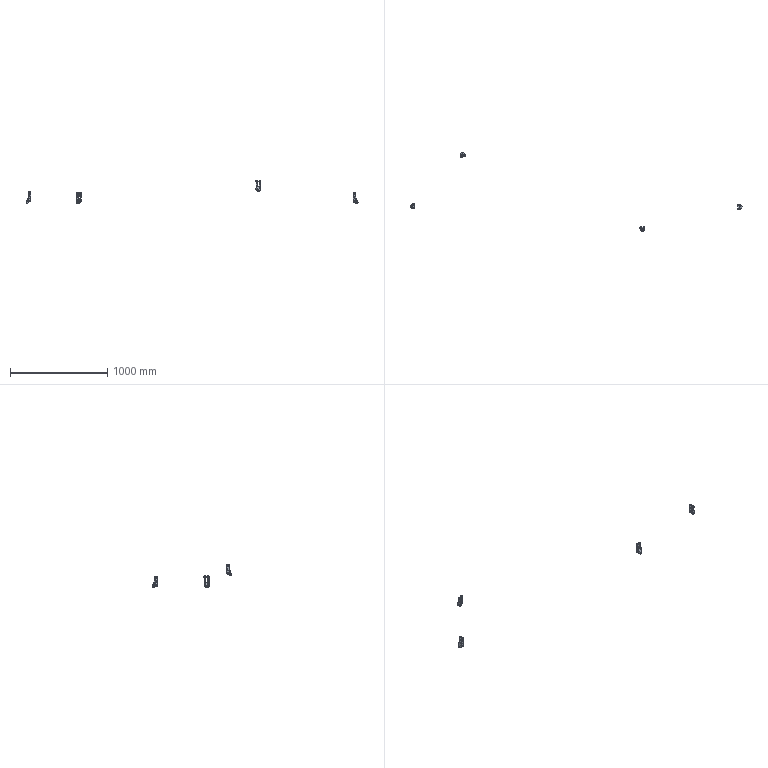Part | STEP file | COMERCIAL_DESTACO_GU5D-04 | 4 solids | 536 faces | box 3406 x 811.269 x 242.561 mm | volume 328941 mm3 | cylinder 248 | plane 208 | cone 80 | commonest cylinder face diameters 3.2 x60 9.5 x56 22.2 x44 6 x24 12.75 x16 14 x16